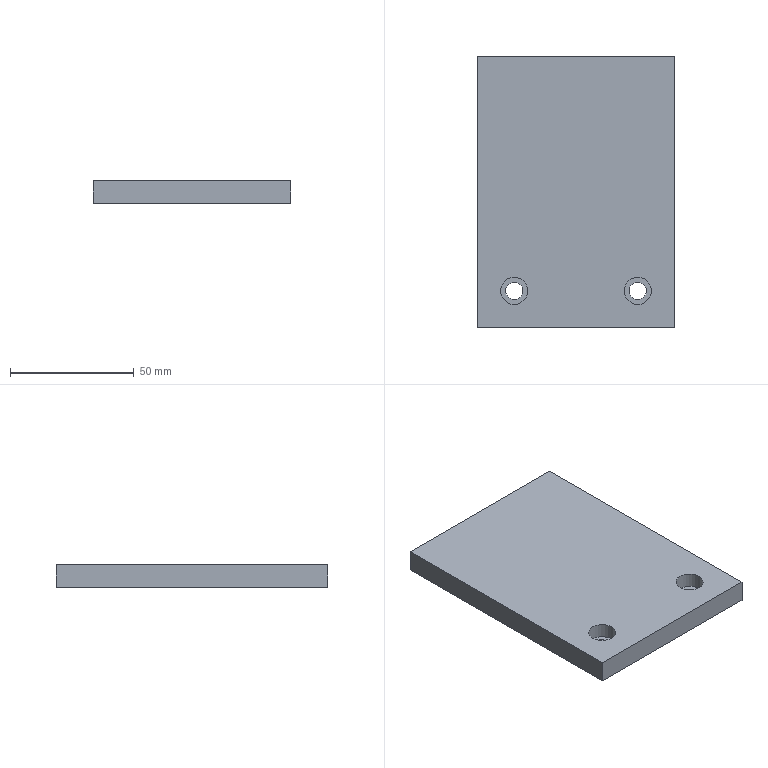Part | NX | features solid 2 | 1 solid | 12 faces | box 80 x 110 x 9 mm | volume 77829 mm3 | plane 8 | cylinder 4 | commonest cylinder face diameters 7 x2 11 x2
STEP:
#1=CARTESIAN_POINT('',(250.,-158.5,361.));
#2=VERTEX_POINT('',#1);
#3=CARTESIAN_POINT('',(250.,-155.,361.));
#4=DIRECTION('',(0.,0.,1.));
#5=DIRECTION('',(0.,-1.,0.));
#6=AXIS2_PLACEMENT_3D('',#3,#4,#5);
#7=CIRCLE('',#6,3.5);
#8=EDGE_CURVE('',#2,#2,#7,.T.);
#9=ORIENTED_EDGE('',*,*,#8,.T.);
#10=EDGE_LOOP('',(#9));
#11=FACE_BOUND('',#10,.T.);
#12=CARTESIAN_POINT('',(200.,-158.5,361.));
#13=VERTEX_POINT('',#12);
#14=CARTESIAN_POINT('',(200.,-155.,361.));
#15=DIRECTION('',(0.,0.,1.));
#16=DIRECTION('',(0.,-1.,0.));
#17=AXIS2_PLACEMENT_3D('',#14,#15,#16);
#18=CIRCLE('',#17,3.5);
#19=EDGE_CURVE('',#13,#13,#18,.T.);
#20=ORIENTED_EDGE('',*,*,#19,.T.);
#21=EDGE_LOOP('',(#20));
#22=FACE_BOUND('',#21,.T.);
#23=CARTESIAN_POINT('',(185.,-60.,361.));
#24=VERTEX_POINT('',#23);
#25=CARTESIAN_POINT('',(185.,-170.,361.));
#26=VERTEX_POINT('',#25);
#27=CARTESIAN_POINT('',(185.,-160.,361.));
#28=DIRECTION('',(0.,-1.,0.));
#29=VECTOR('',#28,1000.);
#30=LINE('',#27,#29);
#31=EDGE_CURVE('',#24,#26,#30,.T.);
#32=ORIENTED_EDGE('',*,*,#31,.F.);
#33=CARTESIAN_POINT('',(265.,-60.,361.));
#34=VERTEX_POINT('',#33);
#35=CARTESIAN_POINT('',(195.,-60.,361.));
#36=DIRECTION('',(-1.,0.,0.));
#37=VECTOR('',#36,1000.);
#38=LINE('',#35,#37);
#39=EDGE_CURVE('',#34,#24,#38,.T.);
#40=ORIENTED_EDGE('',*,*,#39,.F.);
#41=CARTESIAN_POINT('',(265.,-170.,361.));
#42=VERTEX_POINT('',#41);
#43=CARTESIAN_POINT('',(265.,-100.,361.));
#44=DIRECTION('',(0.,1.,0.));
#45=VECTOR('',#44,1000.);
#46=LINE('',#43,#45);
#47=EDGE_CURVE('',#42,#34,#46,.T.);
#48=ORIENTED_EDGE('',*,*,#47,.F.);
#49=CARTESIAN_POINT('',(275.,-170.,361.));
#50=DIRECTION('',(1.,0.,0.));
#51=VECTOR('',#50,1000.);
#52=LINE('',#49,#51);
#53=EDGE_CURVE('',#26,#42,#52,.T.);
#54=ORIENTED_EDGE('',*,*,#53,.F.);
#55=EDGE_LOOP('',(#32,#40,#48,#54));
#56=FACE_BOUND('',#55,.T.);
#57=CARTESIAN_POINT('',(225.,-112.5,361.));
#58=DIRECTION('',(0.,0.,1.));
#59=DIRECTION('',(0.,-1.,0.));
#60=AXIS2_PLACEMENT_3D('',#57,#58,#59);
#61=PLANE('',#60);
#62=ADVANCED_FACE('',(#11,#22,#56),#61,.F.);
#63=CARTESIAN_POINT('',(185.,-60.,370.));
#64=VERTEX_POINT('',#63);
#65=CARTESIAN_POINT('',(185.,-60.,-585.));
#66=DIRECTION('',(0.,0.,1.));
#67=VECTOR('',#66,1000.);
#68=LINE('',#65,#67);
#69=EDGE_CURVE('',#24,#64,#68,.T.);
#70=ORIENTED_EDGE('',*,*,#69,.F.);
#71=ORIENTED_EDGE('',*,*,#31,.T.);
#72=CARTESIAN_POINT('',(185.,-170.,370.));
#73=VERTEX_POINT('',#72);
#74=CARTESIAN_POINT('',(185.,-170.,-85.));
#75=DIRECTION('',(0.,0.,-1.));
#76=VECTOR('',#75,1000.);
#77=LINE('',#74,#76);
#78=EDGE_CURVE('',#73,#26,#77,.T.);
#79=ORIENTED_EDGE('',*,*,#78,.F.);
#80=CARTESIAN_POINT('',(185.,1090.038,370.));
#81=DIRECTION('',(0.,-1.,0.));
#82=VECTOR('',#81,1000.);
#83=LINE('',#80,#82);
#84=EDGE_CURVE('',#64,#73,#83,.T.);
#85=ORIENTED_EDGE('',*,*,#84,.F.);
#86=EDGE_LOOP('',(#70,#71,#79,#85));
#87=FACE_BOUND('',#86,.T.);
#88=CARTESIAN_POINT('',(185.,-160.,-585.));
#89=DIRECTION('',(1.,0.,0.));
#90=DIRECTION('',(0.,0.,1.));
#91=AXIS2_PLACEMENT_3D('',#88,#89,#90);
#92=PLANE('',#91);
#93=ADVANCED_FACE('',(#87),#92,.F.);
#94=CARTESIAN_POINT('',(265.,-60.,370.));
#95=VERTEX_POINT('',#94);
#96=CARTESIAN_POINT('',(265.,-60.,-585.));
#97=DIRECTION('',(0.,0.,-1.));
#98=VECTOR('',#97,1000.);
#99=LINE('',#96,#98);
#100=EDGE_CURVE('',#95,#34,#99,.T.);
#101=ORIENTED_EDGE('',*,*,#100,.T.);
#102=ORIENTED_EDGE('',*,*,#39,.T.);
#103=ORIENTED_EDGE('',*,*,#69,.T.);
#104=CARTESIAN_POINT('',(195.,-60.,370.));
#105=DIRECTION('',(1.,0.,0.));
#106=VECTOR('',#105,1000.);
#107=LINE('',#104,#106);
#108=EDGE_CURVE('',#64,#95,#107,.T.);
#109=ORIENTED_EDGE('',*,*,#108,.T.);
#110=EDGE_LOOP('',(#101,#102,#103,#109));
#111=FACE_BOUND('',#110,.T.);
#112=CARTESIAN_POINT('',(195.,-60.,-585.));
#113=DIRECTION('',(0.,-1.,0.));
#114=DIRECTION('',(0.,0.,-1.));
#115=AXIS2_PLACEMENT_3D('',#112,#113,#114);
#116=PLANE('',#115);
#117=ADVANCED_FACE('',(#111),#116,.F.);
#118=CARTESIAN_POINT('',(265.,-170.,370.));
#119=VERTEX_POINT('',#118);
#120=CARTESIAN_POINT('',(265.,-170.,-85.));
#121=DIRECTION('',(0.,0.,1.));
#122=VECTOR('',#121,1000.);
#123=LINE('',#120,#122);
#124=EDGE_CURVE('',#42,#119,#123,.T.);
#125=ORIENTED_EDGE('',*,*,#124,.F.);
#126=ORIENTED_EDGE('',*,*,#47,.T.);
#127=ORIENTED_EDGE('',*,*,#100,.F.);
#128=CARTESIAN_POINT('',(265.,-100.,370.));
#129=DIRECTION('',(0.,-1.,0.));
#130=VECTOR('',#129,1000.);
#131=LINE('',#128,#130);
#132=EDGE_CURVE('',#95,#119,#131,.T.);
#133=ORIENTED_EDGE('',*,*,#132,.T.);
#134=EDGE_LOOP('',(#125,#126,#127,#133));
#135=FACE_BOUND('',#134,.T.);
#136=CARTESIAN_POINT('',(265.,-100.,-585.));
#137=DIRECTION('',(-1.,0.,0.));
#138=DIRECTION('',(0.,0.,-1.));
#139=AXIS2_PLACEMENT_3D('',#136,#137,#138);
#140=PLANE('',#139);
#141=ADVANCED_FACE('',(#135),#140,.F.);
#142=CARTESIAN_POINT('',(250.,-149.5,370.));
#143=VERTEX_POINT('',#142);
#144=CARTESIAN_POINT('',(250.,-155.,370.));
#145=DIRECTION('',(0.,0.,-1.));
#146=DIRECTION('',(0.,1.,0.));
#147=AXIS2_PLACEMENT_3D('',#144,#145,#146);
#148=CIRCLE('',#147,5.5);
#149=EDGE_CURVE('',#143,#143,#148,.T.);
#150=ORIENTED_EDGE('',*,*,#149,.T.);
#151=EDGE_LOOP('',(#150));
#152=FACE_BOUND('',#151,.T.);
#153=CARTESIAN_POINT('',(200.,-149.5,370.));
#154=VERTEX_POINT('',#153);
#155=CARTESIAN_POINT('',(200.,-155.,370.));
#156=DIRECTION('',(0.,0.,-1.));
#157=DIRECTION('',(0.,1.,0.));
#158=AXIS2_PLACEMENT_3D('',#155,#156,#157);
#159=CIRCLE('',#158,5.5);
#160=EDGE_CURVE('',#154,#154,#159,.T.);
#161=ORIENTED_EDGE('',*,*,#160,.T.);
#162=EDGE_LOOP('',(#161));
#163=FACE_BOUND('',#162,.T.);
#164=CARTESIAN_POINT('',(1450.,-170.,370.));
#165=DIRECTION('',(1.,0.,0.));
#166=VECTOR('',#165,1000.);
#167=LINE('',#164,#166);
#168=EDGE_CURVE('',#73,#119,#167,.T.);
#169=ORIENTED_EDGE('',*,*,#168,.T.);
#170=ORIENTED_EDGE('',*,*,#132,.F.);
#171=ORIENTED_EDGE('',*,*,#108,.F.);
#172=ORIENTED_EDGE('',*,*,#84,.T.);
#173=EDGE_LOOP('',(#169,#170,#171,#172));
#174=FACE_BOUND('',#173,.T.);
#175=CARTESIAN_POINT('',(1450.,1090.038,370.));
#176=DIRECTION('',(0.,0.,-1.));
#177=DIRECTION('',(0.,1.,0.));
#178=AXIS2_PLACEMENT_3D('',#175,#176,#177);
#179=PLANE('',#178);
#180=ADVANCED_FACE('',(#152,#163,#174),#179,.F.);
#181=ORIENTED_EDGE('',*,*,#78,.T.);
#182=ORIENTED_EDGE('',*,*,#53,.T.);
#183=ORIENTED_EDGE('',*,*,#124,.T.);
#184=ORIENTED_EDGE('',*,*,#168,.F.);
#185=EDGE_LOOP('',(#181,#182,#183,#184));
#186=FACE_BOUND('',#185,.T.);
#187=CARTESIAN_POINT('',(275.,-170.,-85.));
#188=DIRECTION('',(0.,1.,0.));
#189=DIRECTION('',(0.,0.,1.));
#190=AXIS2_PLACEMENT_3D('',#187,#188,#189);
#191=PLANE('',#190);
#192=ADVANCED_FACE('',(#186),#191,.F.);
#193=CARTESIAN_POINT('',(200.,-151.5,364.));
#194=VERTEX_POINT('',#193);
#195=CARTESIAN_POINT('',(200.,-155.,364.));
#196=DIRECTION('',(0.,0.,-1.));
#197=DIRECTION('',(0.,1.,0.));
#198=AXIS2_PLACEMENT_3D('',#195,#196,#197);
#199=CIRCLE('',#198,3.5);
#200=EDGE_CURVE('',#194,#194,#199,.T.);
#201=ORIENTED_EDGE('',*,*,#200,.F.);
#202=EDGE_LOOP('',(#201));
#203=FACE_BOUND('',#202,.T.);
#204=ORIENTED_EDGE('',*,*,#19,.F.);
#205=EDGE_LOOP('',(#204));
#206=FACE_BOUND('',#205,.T.);
#207=CARTESIAN_POINT('',(200.,-155.,320.));
#208=DIRECTION('',(0.,0.,-1.));
#209=DIRECTION('',(0.,1.,0.));
#210=AXIS2_PLACEMENT_3D('',#207,#208,#209);
#211=CYLINDRICAL_SURFACE('',#210,3.5);
#212=ADVANCED_FACE('',(#203,#206),#211,.F.);
#213=ORIENTED_EDGE('',*,*,#200,.T.);
#214=EDGE_LOOP('',(#213));
#215=FACE_BOUND('',#214,.T.);
#216=CARTESIAN_POINT('',(200.,-149.5,364.));
#217=VERTEX_POINT('',#216);
#218=CARTESIAN_POINT('',(200.,-155.,364.));
#219=DIRECTION('',(0.,0.,-1.));
#220=DIRECTION('',(0.,1.,0.));
#221=AXIS2_PLACEMENT_3D('',#218,#219,#220);
#222=CIRCLE('',#221,5.5);
#223=EDGE_CURVE('',#217,#217,#222,.T.);
#224=ORIENTED_EDGE('',*,*,#223,.F.);
#225=EDGE_LOOP('',(#224));
#226=FACE_BOUND('',#225,.T.);
#227=CARTESIAN_POINT('',(200.,-155.,364.));
#228=DIRECTION('',(0.,0.,-1.));
#229=DIRECTION('',(0.,1.,0.));
#230=AXIS2_PLACEMENT_3D('',#227,#228,#229);
#231=PLANE('',#230);
#232=ADVANCED_FACE('',(#215,#226),#231,.F.);
#233=ORIENTED_EDGE('',*,*,#223,.T.);
#234=EDGE_LOOP('',(#233));
#235=FACE_BOUND('',#234,.T.);
#236=ORIENTED_EDGE('',*,*,#160,.F.);
#237=EDGE_LOOP('',(#236));
#238=FACE_BOUND('',#237,.T.);
#239=CARTESIAN_POINT('',(200.,-155.,370.));
#240=DIRECTION('',(0.,0.,-1.));
#241=DIRECTION('',(0.,1.,0.));
#242=AXIS2_PLACEMENT_3D('',#239,#240,#241);
#243=CYLINDRICAL_SURFACE('',#242,5.5);
#244=ADVANCED_FACE('',(#235,#238),#243,.F.);
#245=CARTESIAN_POINT('',(250.,-151.5,364.));
#246=VERTEX_POINT('',#245);
#247=CARTESIAN_POINT('',(250.,-155.,364.));
#248=DIRECTION('',(0.,0.,-1.));
#249=DIRECTION('',(0.,1.,0.));
#250=AXIS2_PLACEMENT_3D('',#247,#248,#249);
#251=CIRCLE('',#250,3.5);
#252=EDGE_CURVE('',#246,#246,#251,.T.);
#253=ORIENTED_EDGE('',*,*,#252,.F.);
#254=EDGE_LOOP('',(#253));
#255=FACE_BOUND('',#254,.T.);
#256=ORIENTED_EDGE('',*,*,#8,.F.);
#257=EDGE_LOOP('',(#256));
#258=FACE_BOUND('',#257,.T.);
#259=CARTESIAN_POINT('',(250.,-155.,320.));
#260=DIRECTION('',(0.,0.,-1.));
#261=DIRECTION('',(0.,1.,0.));
#262=AXIS2_PLACEMENT_3D('',#259,#260,#261);
#263=CYLINDRICAL_SURFACE('',#262,3.5);
#264=ADVANCED_FACE('',(#255,#258),#263,.F.);
#265=ORIENTED_EDGE('',*,*,#252,.T.);
#266=EDGE_LOOP('',(#265));
#267=FACE_BOUND('',#266,.T.);
#268=CARTESIAN_POINT('',(250.,-149.5,364.));
#269=VERTEX_POINT('',#268);
#270=CARTESIAN_POINT('',(250.,-155.,364.));
#271=DIRECTION('',(0.,0.,-1.));
#272=DIRECTION('',(0.,1.,0.));
#273=AXIS2_PLACEMENT_3D('',#270,#271,#272);
#274=CIRCLE('',#273,5.5);
#275=EDGE_CURVE('',#269,#269,#274,.T.);
#276=ORIENTED_EDGE('',*,*,#275,.F.);
#277=EDGE_LOOP('',(#276));
#278=FACE_BOUND('',#277,.T.);
#279=CARTESIAN_POINT('',(250.,-155.,364.));
#280=DIRECTION('',(0.,0.,-1.));
#281=DIRECTION('',(0.,1.,0.));
#282=AXIS2_PLACEMENT_3D('',#279,#280,#281);
#283=PLANE('',#282);
#284=ADVANCED_FACE('',(#267,#278),#283,.F.);
#285=ORIENTED_EDGE('',*,*,#275,.T.);
#286=EDGE_LOOP('',(#285));
#287=FACE_BOUND('',#286,.T.);
#288=ORIENTED_EDGE('',*,*,#149,.F.);
#289=EDGE_LOOP('',(#288));
#290=FACE_BOUND('',#289,.T.);
#291=CARTESIAN_POINT('',(250.,-155.,370.));
#292=DIRECTION('',(0.,0.,-1.));
#293=DIRECTION('',(0.,1.,0.));
#294=AXIS2_PLACEMENT_3D('',#291,#292,#293);
#295=CYLINDRICAL_SURFACE('',#294,5.5);
#296=ADVANCED_FACE('',(#287,#290),#295,.F.);
#297=CLOSED_SHELL('',(#62,#93,#117,#141,#180,#192,#212,#232,#244,#264,#284,#296));
#298=MANIFOLD_SOLID_BREP('',#297);
#299=(LENGTH_UNIT()NAMED_UNIT(*)SI_UNIT(.MILLI.,.METRE.));
#300=UNCERTAINTY_MEASURE_WITH_UNIT(LENGTH_MEASURE(0.00001),#299,'','');
#301=(NAMED_UNIT(*)PLANE_ANGLE_UNIT()SI_UNIT($,.RADIAN.));
#302=(NAMED_UNIT(*)SI_UNIT($,.STERADIAN.)SOLID_ANGLE_UNIT());
#303=(GEOMETRIC_REPRESENTATION_CONTEXT(3)GLOBAL_UNCERTAINTY_ASSIGNED_CONTEXT((#300))GLOBAL_UNIT_ASSIGNED_CONTEXT((#299,#301,#302))REPRESENTATION_CONTEXT('',''));
#304=ADVANCED_BREP_SHAPE_REPRESENTATION('',(#298),#303);